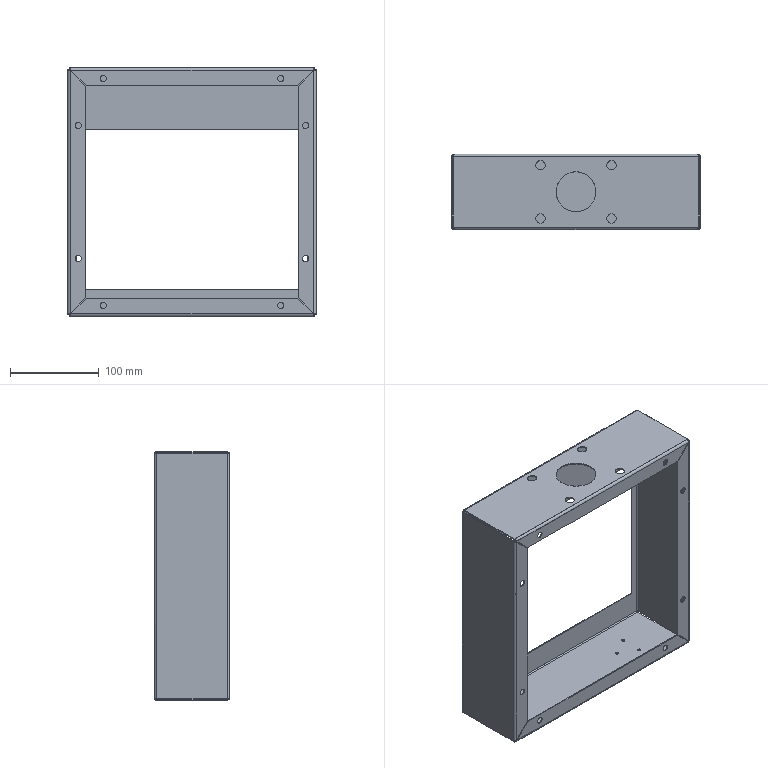Part | STEP file | JBJ-P-1013-01 | 1 solid | 90 faces | box 280 x 85 x 280 mm | volume 166865 mm3 | plane 42 | cylinder 32 | spline 16 | commonest cylinder face diameters 3 x8 5.4 x8 7 x8 10.5 x4 3.5 x3 45 x1